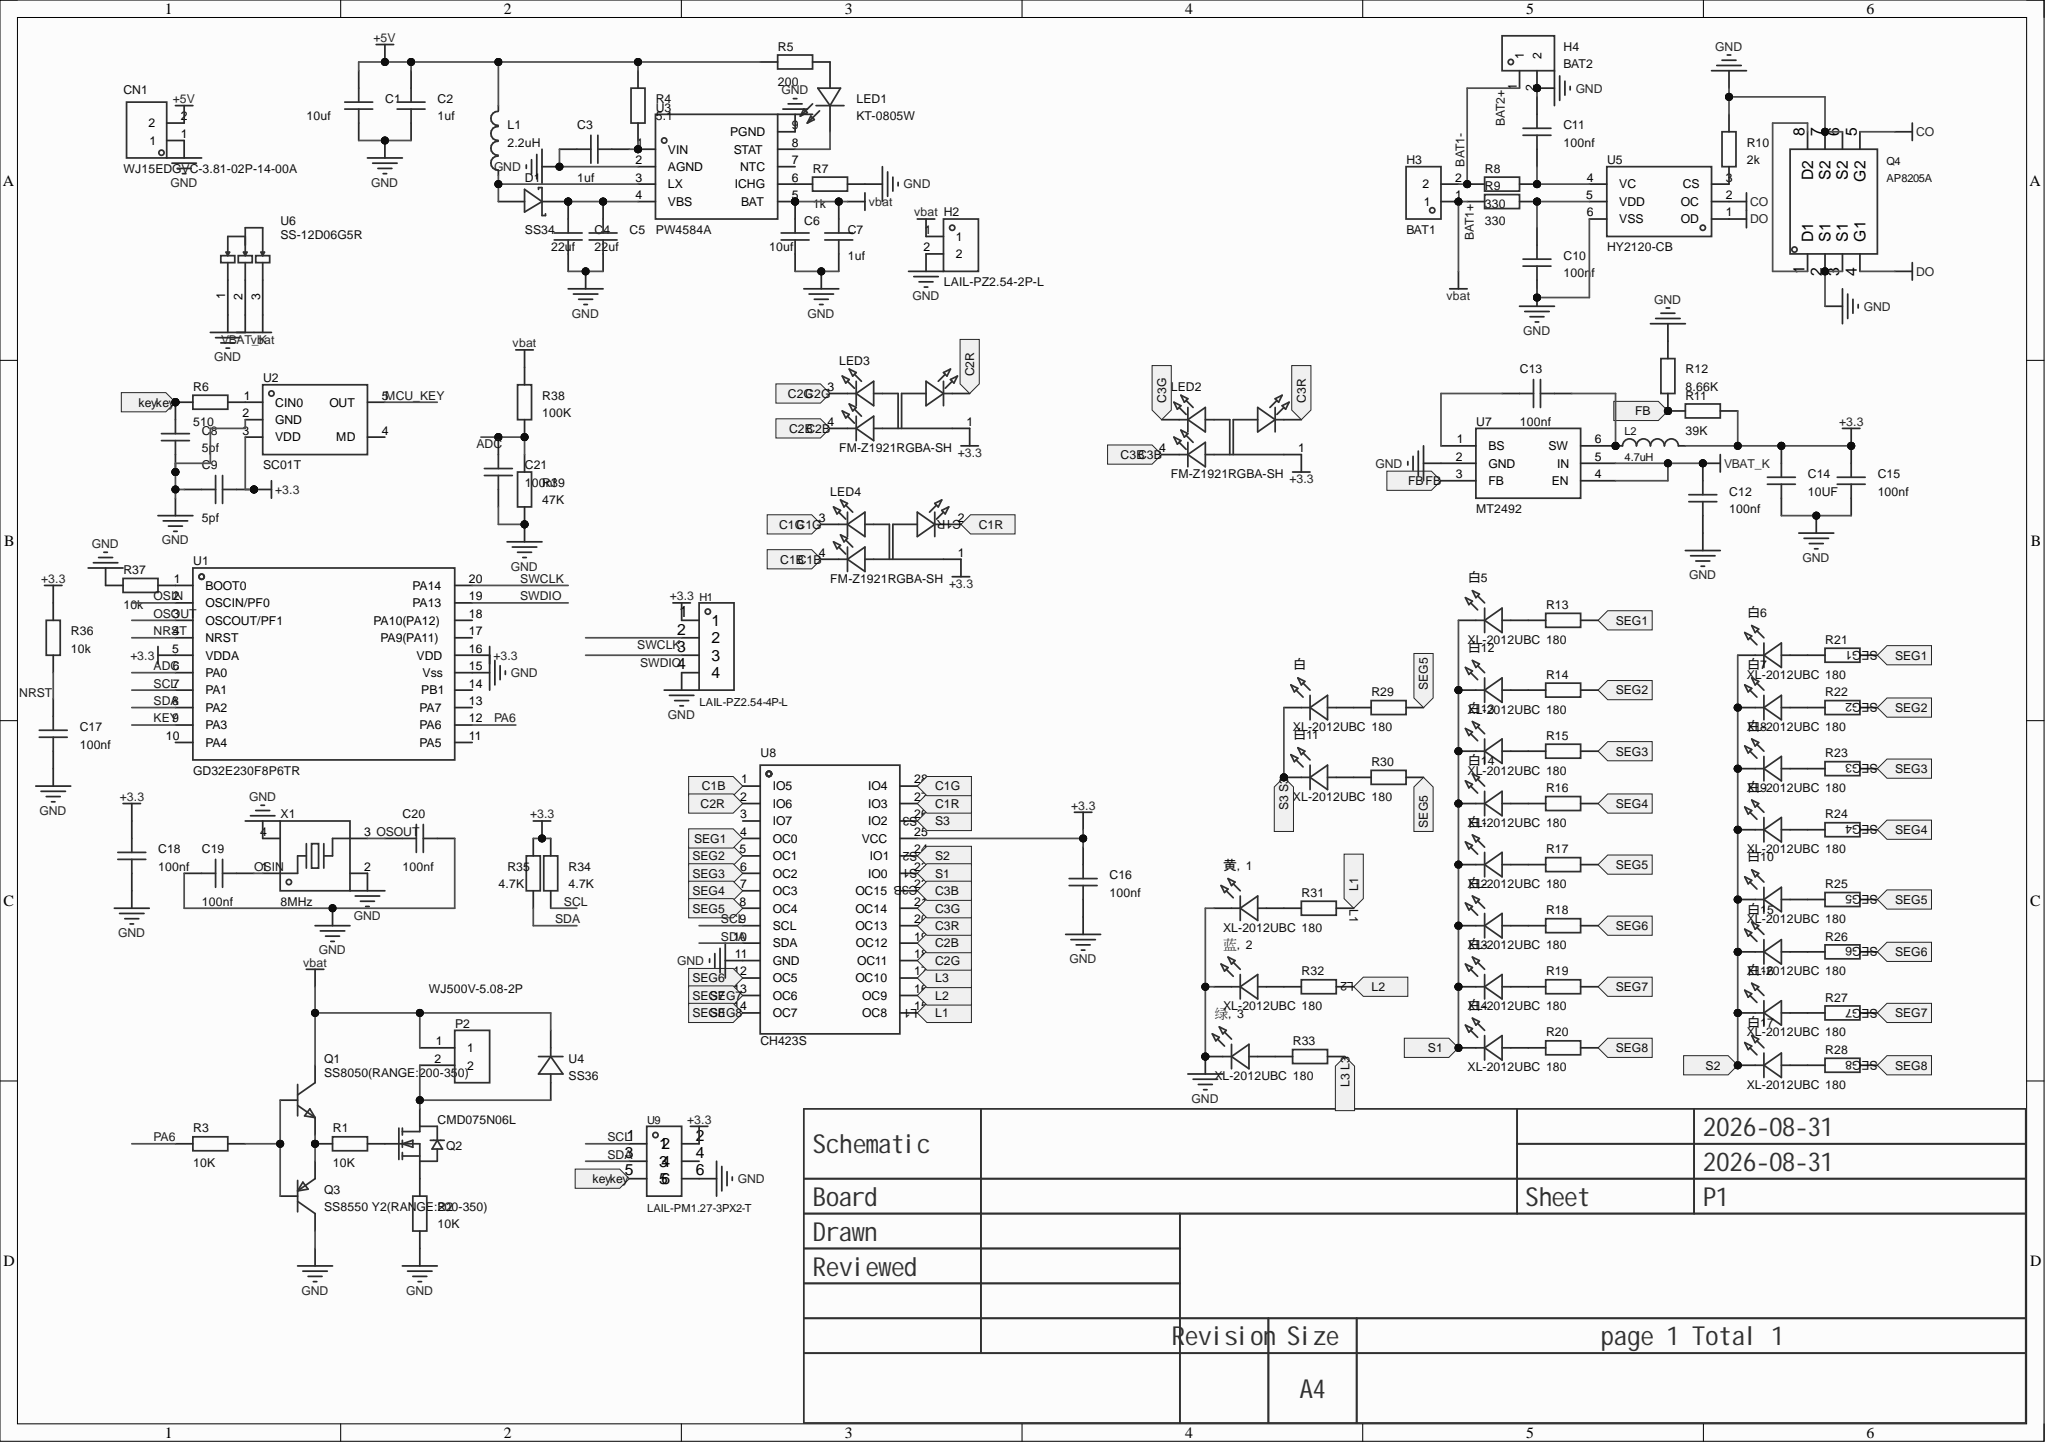Circuit board | Altium Designer | 108 parts | 82 nets
Bill of materials:
Comment,Description,Designator,Footprint,LibRef,Quantity
"10uf","","C1, C6, C14","C0603","CAP_0603","3"
"1uf","","C2, C3, C7","C0603","CAP_0603","3"
"22uf","","C4, C5","C0603","CAP_0603","2"
"5pf","","C8, C9","C0603","CAP_0603","2"
"100nf","","C10, C11, C12, C13, C15, C16, C17, C18, C19, C20, C21","C0603","CAP_0603","11"
"WJ15EDGVC-3.81-02P-14-00A","连接器类型:板端/插座-闭口;固定方式:无固定装置;结构:1x2P;间距:3.81mm;颜色:绿色;安装方式:直插;排数:1;每排PIN数:2;额定电流:8A;额定电压:300V;线规 - AWG:-;线规 - 平方毫米:-;工作温度:-40℃~+105℃;","CN1","CONN-TH_WJ15EDGVC-3.81-2P","WJ15EDGVC-3.81-02P-14-00A","1"
"SS34","Diode configuration: single; forward voltage (Vf): 550mV@3A; DC reverse voltage (Vr): 40V; rectified current: 3A;","D1","SMA_L4.3-W2.6-LS5.2-RD","SS34_C8678","1"
"LAIL-PZ2.54-4P-L","Pin structure: 1x4P; pitch: 2.54mm; round/square pin: square pin; rows: single row; total pin positions: 4P; rated current: 3A; rated voltage: 250V; plastic height: 2.5mm; tail length: 3mm; contact material: brass; contact plating: gold; operating temperature: -25℃~+80℃; color: black;","H1","CONN-TH_LAIL-PZ2.54-4P-L","LAIL-PZ2.54-4P-L","1"
"LAIL-PZ2.54-2P-L","Pin structure: 1x2P; pitch: 2.54mm; round/square pin: square pin; rows: single row; total pin positions: 2P; rated current: 3A; rated voltage: 250V; plastic height: 2.5mm; tail length: 3mm; contact material: brass; contact plating: gold; operating temperature: -25℃~+80℃; color: black;","H2","CONN-TH_LAIL-PZ2.54-2P-L","LAIL-PZ2.54-2P-L","1"
"BAT1","Pin structure: 1x2P; pitch: 2.54mm; round/square pin: square pin; rows: single row; total pin positions: 2P; rated current: 3A; rated voltage: 250V; plastic height: 2.5mm; tail length: 3mm; contact material: brass; contact plating: gold; operating temperature: -25℃~+80℃; color: black;","H3","CONN-TH_LAIL-PZ2.54-2P-L","LAIL-PZ2.54-2P-L","1"
"BAT2","Pin structure: 1x2P; pitch: 2.54mm; round/square pin: square pin; rows: single row; total pin positions: 2P; rated current: 3A; rated voltage: 250V; plastic height: 2.5mm; tail length: 3mm; contact material: brass; contact plating: gold; operating temperature: -25℃~+80℃; color: black;","H4","CONN-TH_LAIL-PZ2.54-2P-L","LAIL-PZ2.54-2P-L","1"
"2.2uH","Inductance: 2.2uH; tolerance: ±20%; rated current: 3.4A; saturation current (Isat): 3.4A;","L1","IND-SMD_L4.0-W4.0_LQH44PN2R2MP0L","SMNR4020-2.2UH","1"
"4.7uH","Inductance: 4.7uH; tolerance: ±20%; rated current: 2.3A; saturation current (Isat): 3.2A; type: magnetic-glue shielded inductor;","L2","IND-SMD_L4.0-W4.0_SMNR4012","PNR4030-4R7-M","1"
"KT-0805W","Lamp holder type: 2mmx1.25mm square holder; illumination color: white; forward voltage (Vf): 2.6V~3.2V; power: 80mW; forward current: 25mA; wavelength: -; diode configuration: single diode; lens color: yellow lens; color temperature: 13172K~100000K; luminous intensity: 350mcd; viewing angle: 120°; carrier tape: top mount; operating temperature: -30℃~+85℃;","LED1","LED0805-R-RD","KT-0805W","1"
"FM-Z1921RGBA-SH","Outdoor gold-wire RGB, black outside white inside design, high contrast","LED2, LED3, LED4","LED-ARRAY-SMD_4P-L2.2-W2.1-BR","FM-Z1921RGBA-SH","3"
"WJ500V-5.08-2P","结构:1x2P;间距:5.08mm;颜色:绿色;安装类型:直插;排数:1;每排PIN数:2;额定电流:18A;额定电压:250V;线规 - AWG:14~30;线规 - 平方毫米:2.5;工作温度:-40℃~+105℃;","P2","CONN-TH_2P-P5.00_WJ500V-5.08-2P","WJ500V-5.08-2P","1"
"SS8050(RANGE:200-350)","Transistor type: NPN; collector current (Ic): 1.5A; collector-emitter breakdown voltage (Vceo): 25V; power dissipation (Pd): 300mW; DC current gain (hFE): 200@800mA,1V;","Q1","SOT-23-3_L2.9-W1.3-P1.90-LS2.4-BR","SS8050(RANGE:200-350)_C2150","1"
"CMD075N06L","MOS管,封装：TO-252，电压：60V,电流：90A,10V内阻：0.0075欧，4.5V内阻：0.011欧，功率：130W，Cisstyp:2100pF","Q2","TO-252-2_L6.6-W6.1-P4.57-LS9.9-BR-CW","CMD075N06L","1"
"SS8550 Y2(RANGE:200-350)","Transistor type: PNP; collector current (Ic): 1.5A; collector-emitter breakdown voltage (Vceo): 25V; power (Pd): 300mW; DC current gain (hFE@Ic,Vce): 200@100mA,1V;","Q3","SOT-23-3_L2.9-W1.3-P1.90-LS2.4-BR","SS8550 Y2(RANGE:200-350)","1"
"AP8205A","Quantity: 2 N-channel; drain-source voltage (Vdss): 20V; continuous drain current (Id): 6A; on-resistance (RDS(on)): 36mO@2.5V; power dissipation (Pd): 1.5W; threshold voltage (Vgs(th)): 1.2V;","Q4","TSSOP-8_L4.4-W3.0-P0.65-LS6.4-BL-2","AP8205A","1"
"10K","","R1, R2, R3, R36, R37","R0603","Res_0603","5"
"5.1","","R4","R0603","Res_0603","1"
"200","","R5","R0603","Res_0603","1"
"510","","R6","R0603","Res_0603","1"
"1k","","R7","R0603","Res_0603","1"
"330","","R8, R9","R0603","Res_0603","2"
"2k","","R10","R0603","Res_0603","1"
"39K","","R11","R0603","Res_0603","1"
"8.66K","","R12","R0603","Res_0603","1"
"180","","R13, R14, R15, R16, R17, R18, R19, R20, R21, R22, R23, R24, R25, R26, R27, R28, R29, R30, R31, R32, R33","R0603","Res_0603","21"
"4.7K","","R34, R35","R0603","Res_0603","2"
"100K","","R38","R0603","Res_0603","1"
"47K","","R39","R0603","Res_0603","1"
"GD32E230F8P6TR","CPU core: ARM Cortex-M series; max CPU frequency: 72MHz;","U1","TSSOP-20_L6.5-W4.4-P0.65-LS6.4-BL","GD32E230F8P6TR","1"
"SC01T","Channels: 1; features: capacitive touch; automatic sensitivity calibration; self-locking: yes;","U2","SOT-23-5_L2.9-W1.6-P0.95-LS2.8-BR","SC01T","1"
"PW4584A","","U3","ESOP-8_L4.9-W3.9-P1.27-LS6.0-BL-EP-1","PW4584A","1"
"SS36","","U4","SMA_L4.3-W2.6-LS5.1-RD","SS36","1"
"HY2120-CB","Operating voltage: 1.5V~10V; max charge current: -; battery type: lithium battery; battery cells: 2;","U5","SOT-23-6_L2.9-W1.6-P0.95-LS2.8-BR","HY2120-CB","1"
"SS-12D06G5R","电路结构:单刀双掷;安装方式:弯插;开关颜色:红色;额定电流:3A;额定电压:125V;工作寿命:1万次;","U6","SW-TH_SS-12D06G5R","SS-12D06G5R","1"
"MT2492","Function type: step-down; operating voltage: 4.5V~16V; output voltage: -; output current: 2A; output type: adjustable;","U7","SOT-23-6_L2.9-W1.6-P0.95-LS2.8-BL_3","MT2492","1"
"CH423S","Interface type: -; I/O count: 8; clock frequency (fc): 1MHz;","U8","SOP-28_L17.9-W7.5-P1.27-LS10.3-BL","CH423S","1"
"LAIL-PM1.27-3PX2-T","Socket structure: 2x3P; pitch: 1.27mm; row spacing: 1.27mm; round/square hole: square hole; rows: double row; total hole positions: 6P; rated current: 1A; rated voltage: 250V; socket direction: top; plastic height: 4.3mm; contact material: phosphor bronze; contact plating: gold; operating temperature: -25℃~+80℃;","U9","HDR-SMD_6P-P1.27_LAIL-PM1.27-3PX2-T","LAIL-PM1.27-3PX2-T","1"
"8MHz","Crystal type: SMD crystal; frequency: 8MHz; frequency deviation at room temperature: ±10ppm; load capacitance: 20pF; frequency stability: ±20ppm;","X1","CRYSTAL-SMD_4P-L3.2-W2.5-BL","XL2EL89CSI-KPIYLC-8M","1"
"XL-2012UBC","Lamp holder type: 2.0mmx1.2mm square holder; illumination color: blue; forward voltage (Vf): 3.2V; power: 70mW; forward current: 20mA; wavelength: 460nm~475nm; diode configuration: single diode; lens color: colorless transparent lens; color temperature: -; luminous intensity: 260mcd; viewing angle: 120°; carrier tape: top mount; operating temperature: -40℃~+85℃;","?, 白1, 白2, 白3, 白4, 白5, 白6, 白7, 白8, 白9, 白10, 白11, 白12, 白13, 白14, 白15, 白16, 白17, ?, 3, ?, 2, ?, 1","LED0805-RD","XL-2012UBC","21"
Netlist (Protel format):
[
C1
C0603
10uf



]
[
C2
C0603
1uf



]
[
C3
C0603
1uf



]
[
C4
C0603
22uf



]
[
C5
C0603
22uf



]
[
C6
C0603
10uf



]
[
C7
C0603
1uf



]
[
C8
C0603
5pf



]
[
C9
C0603
5pf



]
[
C10
C0603
100nf



]
[
C11
C0603
100nf



]
[
C12
C0603
100nf



]
[
C13
C0603
100nf



]
[
C14
C0603
10UF



]
[
C15
C0603
100nf



]
[
C16
C0603
100nf



]
[
C17
C0603
100nf



]
[
C18
C0603
100nf



]
[
C19
C0603
100nf



]
[
C20
C0603
100nf



]
[
C21
C0603
100nf



]
[
CN1
CONN-TH_WJ15EDGVC-3.81-2P
WJ15EDGVC-3.81-02P-14-00A



]
[
D1
SMA_L4.3-W2.6-LS5.2-RD
SS34



]
[
H1
CONN-TH_LAIL-PZ2.54-4P-L
LAIL-PZ2.54-4P-L



]
[
H2
CONN-TH_LAIL-PZ2.54-2P-L
LAIL-PZ2.54-2P-L



]
[
H3
CONN-TH_LAIL-PZ2.54-2P-L
BAT1



]
[
H4
CONN-TH_LAIL-PZ2.54-2P-L
BAT2



]
[
L1
IND-SMD_L4.0-W4.0_LQH44PN2R2MP0L
2.2uH



]
[
L2
IND-SMD_L4.0-W4.0_SMNR4012
4.7uH



]
[
LED1
LED0805-R-RD
KT-0805W



]
[
LED2
LED-ARRAY-SMD_4P-L2.2-W2.1-BR
FM-Z1921RGBA-SH



]
[
LED3
LED-ARRAY-SMD_4P-L2.2-W2.1-BR
FM-Z1921RGBA-SH



]
[
LED4
LED-ARRAY-SMD_4P-L2.2-W2.1-BR
FM-Z1921RGBA-SH



]
[
P2
CONN-TH_2P-P5.00_WJ500V-5.08-2P
WJ500V-5.08-2P



]
[
Q1
SOT-23-3_L2.9-W1.3-P1.90-LS2.4-BR
SS8050(RANGE:200-350)



]
[
Q2
TO-252-2_L6.6-W6.1-P4.57-LS9.9-BR-CW
CMD075N06L



]
[
Q3
SOT-23-3_L2.9-W1.3-P1.90-LS2.4-BR
SS8550 Y2(RANGE:200-350)



]
[
Q4
TSSOP-8_L4.4-W3.0-P0.65-LS6.4-BL-2
AP8205A



]
[
R1
R0603
10K



]
[
R2
R0603
10K



]
[
R3
R0603
10K



]
[
R4
R0603
5.1



]
[
R5
R0603
200



]
[
R6
R0603
510



]
[
R7
R0603
1k



]
[
R8
R0603
330



]
[
R9
R0603
330



]
[
R10
R0603
2k



]
[
R11
R0603
39K



]
[
R12
R0603
8.66K



]
[
R13
R0603
180



]
[
R14
R0603
180



]
[
R15
R0603
180



]
[
R16
R0603
180



]
[
R17
R0603
180



]
[
R18
R0603
180



]
[
R19
R0603
180



]
[
R20
R0603
180



]
[
R21
R0603
180



]
[
R22
R0603
180



]
[
R23
R0603
180



]
[
R24
R0603
180



]
[
R25
R0603
180



]
[
R26
R0603
180



]
[
R27
R0603
180



]
[
R28
R0603
180



]
[
R29
R0603
180



]
[
R30
R0603
180



]
[
R31
R0603
180



]
[
R32
R0603
180



]
[
R33
R0603
180



]
[
R34
R0603
4.7K



]
[
R35
R0603
4.7K



]
[
R36
R0603
10k



]
[
R37
R0603
10k



]
[
R38
R0603
100K



]
[
R39
R0603
47K



]
[
U1
TSSOP-20_L6.5-W4.4-P0.65-LS6.4-BL
GD32E230F8P6TR



]
[
U2
SOT-23-5_L2.9-W1.6-P0.95-LS2.8-BR
SC01T



]
[
U3
ESOP-8_L4.9-W3.9-P1.27-LS6.0-BL-EP-1
PW4584A



]
[
U4
SMA_L4.3-W2.6-LS5.1-RD
SS36



]
[
U5
SOT-23-6_L2.9-W1.6-P0.95-LS2.8-BR
HY2120-CB



]
[
U6
SW-TH_SS-12D06G5R
SS-12D06G5R



]
[
U7
SOT-23-6_L2.9-W1.6-P0.95-LS2.8-BL_3
MT2492



]
[
U8
SOP-28_L17.9-W7.5-P1.27-LS10.3-BL
CH423S



]
[
U9
HDR-SMD_6P-P1.27_LAIL-PM1.27-3PX2-T
LAIL-PM1.27-3PX2-T



]
[
X1
CRYSTAL-SMD_4P-L3.2-W2.5-BL
8MHz



]
[
白
LED0805-RD
XL-2012UBC



]
[
白1
LED0805-RD
XL-2012UBC



]
[
白2
LED0805-RD
XL-2012UBC



]
[
白3
LED0805-RD
XL-2012UBC



]
[
白4
LED0805-RD
XL-2012UBC



]
[
白5
LED0805-RD
XL-2012UBC



]
[
白6
LED0805-RD
XL-2012UBC



]
[
白7
LED0805-RD
XL-2012UBC



]
[
白8
LED0805-RD
XL-2012UBC



]
[
白9
LED0805-RD
XL-2012UBC



]
[
白10
LED0805-RD
XL-2012UBC



]
[
白11
LED0805-RD
XL-2012UBC



]
[
白12
LED0805-RD
XL-2012UBC



]
[
白13
LED0805-RD
XL-2012UBC



]
[
白14
LED0805-RD
XL-2012UBC



]
[
白15
LED0805-RD
XL-2012UBC



]
[
白16
LED0805-RD
XL-2012UBC



]
[
白17
LED0805-RD
XL-2012UBC



]
[
绿，3
LED0805-RD
XL-2012UBC



]
[
蓝，2
LED0805-RD
XL-2012UBC



]
[
黄，1
LED0805-RD
XL-2012UBC



]
(
VBAT_K
C12-2
U6-2
U7-4
U7-5
)
(
SWDIO
H1-3
U1-19
)
(
SWCLK
H1-2
U1-20
)
(
SEG8
R20-1
R28-1
U8-14
)
(
SEG7
R19-1
R27-1
U8-13
)
(
SEG6
R18-1
R26-1
U8-12
)
(
SEG5
R17-1
R25-1
R29-1
R30-1
U8-8
)
(
SEG4
R16-1
R24-1
U8-7
)
(
SEG3
R15-1
R23-1
U8-6
)
(
SEG2
R14-1
R22-1
U8-5
)
(
SEG1
R13-1
R21-1
U8-4
)
(
SDA
R35-1
U1-8
U8-10
U9-3
)
(
SCL
R34-1
U1-7
U8-9
U9-1
)
(
S3
U8-26
白-1
白11-1
)
(
S2
U8-24
白6-1
白7-1
白8-1
白9-1
白10-1
白15-1
白16-1
白17-1
)
(
S1
U8-23
白1-1
白2-1
白3-1
白4-1
白5-1
白12-1
白13-1
白14-1
)
(
PA6
R3-1
U1-12
)
(
OSOUT
C20-1
U1-3
X1-3
)
(
OSIN
C19-1
U1-2
X1-1
)
(
NRST
C17-1
R36-1
U1-4
)
(
NetR37_1
R37-1
U1-1
)
(
NetR33_2
R33-2
绿，3-2
)
(
NetR32_2
R32-2
蓝，2-2
)
(
NetR31_2
R31-2
黄，1-2
)
(
NetR30_2
R30-2
白11-2
)
(
NetR29_2
R29-2
白-2
)
(
NetR28_2
R28-2
白17-2
)
(
NetR27_2
R27-2
白16-2
)
(
NetR26_2
R26-2
白15-2
)
(
NetR25_2
R25-2
白10-2
)
(
NetR24_2
R24-2
白9-2
)
(
NetR23_2
R23-2
白8-2
)
(
NetR22_2
R22-2
白7-2
)
(
NetR21_2
R21-2
白6-2
)
(
NetR20_2
R20-2
白4-2
)
(
NetR19_2
R19-2
白3-2
)
(
NetR18_2
R18-2
白2-2
)
(
NetR17_2
R17-2
白1-2
)
(
NetR16_2
R16-2
白14-2
)
(
NetR15_2
R15-2
白13-2
)
(
NetR14_2
R14-2
白12-2
)
(
NetR13_2
R13-2
白5-2
)
(
NetR10_1
R10-1
U5-3
)
(
NetR7_1
R7-1
U3-6
)
(
NetR6_2
R6-2
U2-1
)
(
NetQ4_1
Q4-1
Q4-8
)
(
NetQ2_3
Q2-3
R2-2
)
(
NetQ2_1
Q2-1
R1-2
)
(
NetQ1_2
Q1-2
Q3-2
R1-1
)
(
NetQ1_1
Q1-1
Q3-1
R3-2
)
(
NetP2_2
P2-2
Q2-2
U4-2
)
(
NetLED3_2
LED3-2
U8-2
)
(
NetLED2_3
LED2-3
U8-21
)
(
NetLED2_2
LED2-2
U8-20
)
(
NetLED1_2
LED1-2
U3-8
)
(
NetLED1_1
LED1-1
R5-1
)
(
NetD1_2
D1-2
L1-1
U3-3
)
(
NetC13_2
C13-2
U7-1
)
(
NetC13_1
C13-1
L2-1
U7-6
)
(
NetC11_1
C11-1
R8-2
U5-4
)
(
NetC10_2
C10-2
R9-2
U5-5
)
(
NetC4_1
C4-1
C5-2
D1-1
U3-4
)
(
NetC3_2
C3-2
R4-1
U3-1
)
(
L3
R33-1
U8-17
)
(
L2
R32-1
U8-16
)
(
L1
R31-1
U8-15
)
(
key
C8-2
R6-1
U1-9
U9-5
)
(
GND
C1-1
C2-1
C3-1
C4-2
C5-1
C6-2
C7-2
C8-1
C9-2
C10-1
C11-2
C12-1
C14-1
C15-1
C16-1
C17-2
C18-2
C19-2
C20-2
C21-2
CN1-1
H1-4
H2-2
H4-2
Q3-3
Q4-2
Q4-3
Q4-6
Q4-7
R2-1
R7-2
R10-2
R12-2
R37-2
R39-1
U1-15
U2-2
U3-2
U3-9
U5-6
U6-1
U7-2
U8-11
U9-6
X1-2
X1-4
绿，3-1
蓝，2-1
黄，1-1
)
(
FB
R11-2
R12-1
U7-3
)
(
DO
Q4-4
U5-1
)
(
CO
Q4-5
U5-2
)
(
C3B
LED2-4
U8-22
)
(
C2G
LED3-3
U8-18
)
(
C2B
LED3-4
U8-19
)
(
C1R
LED4-2
U8-27
)
(
C1G
LED4-3
U8-28
)
(
C1B
LED4-4
U8-1
)
(
BAT1-
H3-2
H4-1
R8-1
)
(
BAT1+
C6-1
C7-1
H2-1
H3-1
P2-1
Q1-3
R9-1
R38-2
U3-5
U4-1
U6-3
)
(
ADC
C21-1
R38-1
R39-2
U1-6
)
(
+5V
C1-2
C2-2
CN1-2
L1-2
R4-2
R5-2
)
(
+3.3
C9-1
C14-2
C15-2
C16-2
C18-1
H1-1
L2-2
LED2-1
LED3-1
LED4-1
R11-1
R34-2
R35-2
R36-2
U1-5
U1-16
U2-3
U8-25
U9-2
)